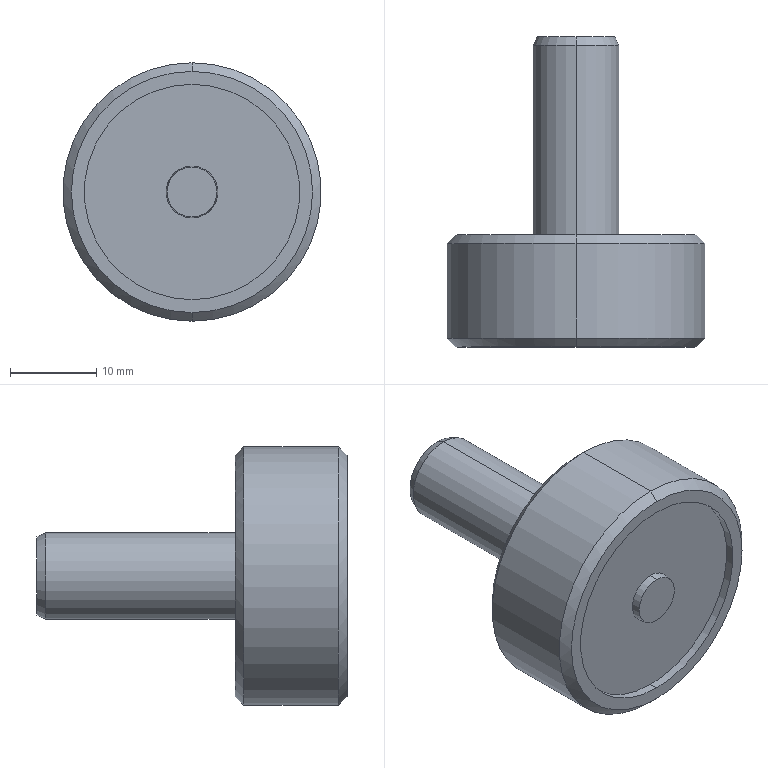Part | SolidWorks | features BaseBody 1 | 1 solid | 19 faces | box 30 x 36 x 30 mm | volume 10433 mm3 | cone 8 | cylinder 6 | plane 5 | commonest cylinder face diameters 10 x2 25 x2 30 x2
STEP:
#1=CARTESIAN_POINT('',(257.5,37.,118.121));
#2=VERTEX_POINT('',#1);
#3=CARTESIAN_POINT('',(257.5,37.,128.121));
#4=VERTEX_POINT('',#3);
#5=CARTESIAN_POINT('',(257.5,37.,123.121));
#6=DIRECTION('',(0.,-1.,0.));
#7=DIRECTION('',(0.,0.,1.));
#8=AXIS2_PLACEMENT_3D('',#5,#6,#7);
#9=CIRCLE('',#8,5.);
#10=EDGE_CURVE('',#2,#4,#9,.T.);
#11=ORIENTED_EDGE('',*,*,#10,.F.);
#12=CARTESIAN_POINT('',(257.5,59.,118.121));
#13=VERTEX_POINT('',#12);
#14=CARTESIAN_POINT('',(257.5,60.,118.121));
#15=DIRECTION('',(0.,1.,0.));
#16=VECTOR('',#15,1000.);
#17=LINE('',#14,#16);
#18=EDGE_CURVE('',#2,#13,#17,.T.);
#19=ORIENTED_EDGE('',*,*,#18,.T.);
#20=CARTESIAN_POINT('',(257.5,59.,128.121));
#21=VERTEX_POINT('',#20);
#22=CARTESIAN_POINT('',(257.5,59.,123.121));
#23=DIRECTION('',(0.,-1.,0.));
#24=DIRECTION('',(0.,0.,1.));
#25=AXIS2_PLACEMENT_3D('',#22,#23,#24);
#26=CIRCLE('',#25,5.);
#27=EDGE_CURVE('',#13,#21,#26,.T.);
#28=ORIENTED_EDGE('',*,*,#27,.T.);
#29=CARTESIAN_POINT('',(257.5,60.,128.121));
#30=DIRECTION('',(0.,1.,0.));
#31=VECTOR('',#30,1000.);
#32=LINE('',#29,#31);
#33=EDGE_CURVE('',#4,#21,#32,.T.);
#34=ORIENTED_EDGE('',*,*,#33,.F.);
#35=EDGE_LOOP('',(#11,#19,#28,#34));
#36=FACE_OUTER_BOUND('',#35,.T.);
#37=CARTESIAN_POINT('',(257.5,60.,123.121));
#38=DIRECTION('',(0.,1.,0.));
#39=DIRECTION('',(0.,0.,1.));
#40=AXIS2_PLACEMENT_3D('',#37,#38,#39);
#41=CYLINDRICAL_SURFACE('',#40,5.);
#42=ADVANCED_FACE('',(#36),#41,.T.);
#43=CARTESIAN_POINT('',(257.5,37.,137.121));
#44=VERTEX_POINT('',#43);
#45=CARTESIAN_POINT('',(257.5,37.,109.121));
#46=VERTEX_POINT('',#45);
#47=CARTESIAN_POINT('',(257.5,37.,123.121));
#48=DIRECTION('',(0.,1.,0.));
#49=DIRECTION('',(0.,0.,-1.));
#50=AXIS2_PLACEMENT_3D('',#47,#48,#49);
#51=CIRCLE('',#50,14.);
#52=EDGE_CURVE('',#44,#46,#51,.T.);
#53=ORIENTED_EDGE('',*,*,#52,.F.);
#54=CARTESIAN_POINT('',(257.5,36.,138.121));
#55=VERTEX_POINT('',#54);
#56=CARTESIAN_POINT('',(257.5,36.,138.121));
#57=DIRECTION('',(0.,-0.7071,0.7071));
#58=VECTOR('',#57,1000.);
#59=LINE('',#56,#58);
#60=EDGE_CURVE('',#44,#55,#59,.T.);
#61=ORIENTED_EDGE('',*,*,#60,.T.);
#62=CARTESIAN_POINT('',(257.5,36.,108.121));
#63=VERTEX_POINT('',#62);
#64=CARTESIAN_POINT('',(257.5,36.,123.121));
#65=DIRECTION('',(0.,1.,0.));
#66=DIRECTION('',(-0.05078,0.,-0.9987));
#67=AXIS2_PLACEMENT_3D('',#64,#65,#66);
#68=CIRCLE('',#67,15.);
#69=EDGE_CURVE('',#55,#63,#68,.T.);
#70=ORIENTED_EDGE('',*,*,#69,.T.);
#71=CARTESIAN_POINT('',(257.5,36.,108.121));
#72=DIRECTION('',(0.,-0.7071,-0.7071));
#73=VECTOR('',#72,1000.);
#74=LINE('',#71,#73);
#75=EDGE_CURVE('',#46,#63,#74,.T.);
#76=ORIENTED_EDGE('',*,*,#75,.F.);
#77=EDGE_LOOP('',(#53,#61,#70,#76));
#78=FACE_OUTER_BOUND('',#77,.T.);
#79=CARTESIAN_POINT('',(257.5,36.,123.121));
#80=DIRECTION('',(0.,-1.,0.));
#81=DIRECTION('',(0.,0.,-1.));
#82=AXIS2_PLACEMENT_3D('',#79,#80,#81);
#83=CONICAL_SURFACE('',#82,15.,0.7854);
#84=ADVANCED_FACE('',(#78),#83,.T.);
#85=CARTESIAN_POINT('',(257.5,60.,118.587));
#86=VERTEX_POINT('',#85);
#87=CARTESIAN_POINT('',(257.5,60.,127.655));
#88=VERTEX_POINT('',#87);
#89=CARTESIAN_POINT('',(257.5,60.,123.121));
#90=DIRECTION('',(0.,-1.,0.));
#91=DIRECTION('',(0.,0.,-1.));
#92=AXIS2_PLACEMENT_3D('',#89,#90,#91);
#93=CIRCLE('',#92,4.534);
#94=EDGE_CURVE('',#86,#88,#93,.T.);
#95=ORIENTED_EDGE('',*,*,#94,.T.);
#96=CARTESIAN_POINT('',(257.5,59.,128.121));
#97=DIRECTION('',(0.,-0.9063,0.4226));
#98=VECTOR('',#97,1000.);
#99=LINE('',#96,#98);
#100=EDGE_CURVE('',#88,#21,#99,.T.);
#101=ORIENTED_EDGE('',*,*,#100,.T.);
#102=ORIENTED_EDGE('',*,*,#27,.F.);
#103=CARTESIAN_POINT('',(257.5,59.,118.121));
#104=DIRECTION('',(0.,-0.9063,-0.4226));
#105=VECTOR('',#104,1000.);
#106=LINE('',#103,#105);
#107=EDGE_CURVE('',#86,#13,#106,.T.);
#108=ORIENTED_EDGE('',*,*,#107,.F.);
#109=EDGE_LOOP('',(#95,#101,#102,#108));
#110=FACE_OUTER_BOUND('',#109,.T.);
#111=CARTESIAN_POINT('',(257.5,59.,123.121));
#112=DIRECTION('',(0.,-1.,0.));
#113=DIRECTION('',(0.,0.,-1.));
#114=AXIS2_PLACEMENT_3D('',#111,#112,#113);
#115=CONICAL_SURFACE('',#114,5.,0.4363);
#116=ADVANCED_FACE('',(#110),#115,.T.);
#117=CARTESIAN_POINT('',(257.5,25.,138.121));
#118=VERTEX_POINT('',#117);
#119=CARTESIAN_POINT('',(257.5,25.,108.121));
#120=VERTEX_POINT('',#119);
#121=CARTESIAN_POINT('',(257.5,25.,123.121));
#122=DIRECTION('',(0.,1.,0.));
#123=DIRECTION('',(0.,0.,1.));
#124=AXIS2_PLACEMENT_3D('',#121,#122,#123);
#125=CIRCLE('',#124,15.);
#126=EDGE_CURVE('',#118,#120,#125,.T.);
#127=ORIENTED_EDGE('',*,*,#126,.T.);
#128=CARTESIAN_POINT('',(257.5,60.,108.121));
#129=DIRECTION('',(0.,1.,0.));
#130=VECTOR('',#129,1000.);
#131=LINE('',#128,#130);
#132=EDGE_CURVE('',#120,#63,#131,.T.);
#133=ORIENTED_EDGE('',*,*,#132,.T.);
#134=ORIENTED_EDGE('',*,*,#69,.F.);
#135=CARTESIAN_POINT('',(257.5,60.,138.121));
#136=DIRECTION('',(0.,1.,0.));
#137=VECTOR('',#136,1000.);
#138=LINE('',#135,#137);
#139=EDGE_CURVE('',#118,#55,#138,.T.);
#140=ORIENTED_EDGE('',*,*,#139,.F.);
#141=EDGE_LOOP('',(#127,#133,#134,#140));
#142=FACE_OUTER_BOUND('',#141,.T.);
#143=CARTESIAN_POINT('',(257.5,60.,123.121));
#144=DIRECTION('',(0.,1.,0.));
#145=DIRECTION('',(0.,0.,1.));
#146=AXIS2_PLACEMENT_3D('',#143,#144,#145);
#147=CYLINDRICAL_SURFACE('',#146,15.);
#148=ADVANCED_FACE('',(#142),#147,.T.);
#149=CARTESIAN_POINT('',(257.5,24.,137.121));
#150=VERTEX_POINT('',#149);
#151=CARTESIAN_POINT('',(257.5,24.,109.121));
#152=VERTEX_POINT('',#151);
#153=CARTESIAN_POINT('',(257.5,24.,123.121));
#154=DIRECTION('',(0.,1.,0.));
#155=DIRECTION('',(0.,0.,1.));
#156=AXIS2_PLACEMENT_3D('',#153,#154,#155);
#157=CIRCLE('',#156,14.);
#158=EDGE_CURVE('',#150,#152,#157,.T.);
#159=ORIENTED_EDGE('',*,*,#158,.T.);
#160=CARTESIAN_POINT('',(257.5,25.,108.121));
#161=DIRECTION('',(0.,0.7071,-0.7071));
#162=VECTOR('',#161,1000.);
#163=LINE('',#160,#162);
#164=EDGE_CURVE('',#152,#120,#163,.T.);
#165=ORIENTED_EDGE('',*,*,#164,.T.);
#166=ORIENTED_EDGE('',*,*,#126,.F.);
#167=CARTESIAN_POINT('',(257.5,25.,138.121));
#168=DIRECTION('',(0.,0.7071,0.7071));
#169=VECTOR('',#168,1000.);
#170=LINE('',#167,#169);
#171=EDGE_CURVE('',#150,#118,#170,.T.);
#172=ORIENTED_EDGE('',*,*,#171,.F.);
#173=EDGE_LOOP('',(#159,#165,#166,#172));
#174=FACE_OUTER_BOUND('',#173,.T.);
#175=CARTESIAN_POINT('',(257.5,25.,123.121));
#176=DIRECTION('',(0.,1.,0.));
#177=DIRECTION('',(0.,0.,1.));
#178=AXIS2_PLACEMENT_3D('',#175,#176,#177);
#179=CONICAL_SURFACE('',#178,15.,0.7854);
#180=ADVANCED_FACE('',(#174),#179,.T.);
#181=CARTESIAN_POINT('',(257.5,25.,135.621));
#182=VERTEX_POINT('',#181);
#183=CARTESIAN_POINT('',(257.5,25.,110.621));
#184=VERTEX_POINT('',#183);
#185=CARTESIAN_POINT('',(257.5,25.,123.121));
#186=DIRECTION('',(0.,-1.,0.));
#187=DIRECTION('',(0.,0.,-1.));
#188=AXIS2_PLACEMENT_3D('',#185,#186,#187);
#189=CIRCLE('',#188,12.5);
#190=EDGE_CURVE('',#182,#184,#189,.T.);
#191=ORIENTED_EDGE('',*,*,#190,.F.);
#192=CARTESIAN_POINT('',(257.5,24.,135.621));
#193=VERTEX_POINT('',#192);
#194=CARTESIAN_POINT('',(257.5,25.,135.621));
#195=DIRECTION('',(0.,-1.,0.));
#196=VECTOR('',#195,1000.);
#197=LINE('',#194,#196);
#198=EDGE_CURVE('',#182,#193,#197,.T.);
#199=ORIENTED_EDGE('',*,*,#198,.T.);
#200=CARTESIAN_POINT('',(257.5,24.,110.621));
#201=VERTEX_POINT('',#200);
#202=CARTESIAN_POINT('',(257.5,24.,123.121));
#203=DIRECTION('',(0.,1.,0.));
#204=DIRECTION('',(0.,0.,-1.));
#205=AXIS2_PLACEMENT_3D('',#202,#203,#204);
#206=CIRCLE('',#205,12.5);
#207=EDGE_CURVE('',#201,#193,#206,.T.);
#208=ORIENTED_EDGE('',*,*,#207,.F.);
#209=CARTESIAN_POINT('',(257.5,25.,110.621));
#210=DIRECTION('',(0.,-1.,0.));
#211=VECTOR('',#210,1000.);
#212=LINE('',#209,#211);
#213=EDGE_CURVE('',#184,#201,#212,.T.);
#214=ORIENTED_EDGE('',*,*,#213,.F.);
#215=EDGE_LOOP('',(#191,#199,#208,#214));
#216=FACE_OUTER_BOUND('',#215,.T.);
#217=CARTESIAN_POINT('',(257.5,25.,123.121));
#218=DIRECTION('',(0.,-1.,0.));
#219=DIRECTION('',(0.,0.,-1.));
#220=AXIS2_PLACEMENT_3D('',#217,#218,#219);
#221=CYLINDRICAL_SURFACE('',#220,12.5);
#222=ADVANCED_FACE('',(#216),#221,.F.);
#223=CARTESIAN_POINT('',(257.5,24.,126.016));
#224=VERTEX_POINT('',#223);
#225=CARTESIAN_POINT('',(257.5,24.,120.226));
#226=VERTEX_POINT('',#225);
#227=CARTESIAN_POINT('',(257.5,24.,123.121));
#228=DIRECTION('',(0.,1.,0.));
#229=DIRECTION('',(0.,0.,1.));
#230=AXIS2_PLACEMENT_3D('',#227,#228,#229);
#231=CIRCLE('',#230,2.895);
#232=EDGE_CURVE('',#224,#226,#231,.T.);
#233=ORIENTED_EDGE('',*,*,#232,.T.);
#234=CARTESIAN_POINT('',(257.5,25.,120.121));
#235=VERTEX_POINT('',#234);
#236=CARTESIAN_POINT('',(257.5,25.,120.121));
#237=DIRECTION('',(0.,0.9945,-0.1045));
#238=VECTOR('',#237,1000.);
#239=LINE('',#236,#238);
#240=EDGE_CURVE('',#226,#235,#239,.T.);
#241=ORIENTED_EDGE('',*,*,#240,.T.);
#242=CARTESIAN_POINT('',(257.5,25.,126.121));
#243=VERTEX_POINT('',#242);
#244=CARTESIAN_POINT('',(257.5,25.,123.121));
#245=DIRECTION('',(0.,1.,0.));
#246=DIRECTION('',(0.,0.,1.));
#247=AXIS2_PLACEMENT_3D('',#244,#245,#246);
#248=CIRCLE('',#247,3.);
#249=EDGE_CURVE('',#243,#235,#248,.T.);
#250=ORIENTED_EDGE('',*,*,#249,.F.);
#251=CARTESIAN_POINT('',(257.5,25.,126.121));
#252=DIRECTION('',(0.,0.9945,0.1045));
#253=VECTOR('',#252,1000.);
#254=LINE('',#251,#253);
#255=EDGE_CURVE('',#224,#243,#254,.T.);
#256=ORIENTED_EDGE('',*,*,#255,.F.);
#257=EDGE_LOOP('',(#233,#241,#250,#256));
#258=FACE_OUTER_BOUND('',#257,.T.);
#259=CARTESIAN_POINT('',(257.5,25.,123.121));
#260=DIRECTION('',(0.,1.,0.));
#261=DIRECTION('',(0.,0.,1.));
#262=AXIS2_PLACEMENT_3D('',#259,#260,#261);
#263=CONICAL_SURFACE('',#262,3.,0.1047);
#264=ADVANCED_FACE('',(#258),#263,.T.);
#265=CARTESIAN_POINT('',(257.5,37.,123.121));
#266=DIRECTION('',(0.,-1.,0.));
#267=DIRECTION('',(0.,0.,1.));
#268=AXIS2_PLACEMENT_3D('',#265,#266,#267);
#269=CIRCLE('',#268,5.);
#270=EDGE_CURVE('',#4,#2,#269,.T.);
#271=ORIENTED_EDGE('',*,*,#270,.T.);
#272=ORIENTED_EDGE('',*,*,#10,.T.);
#273=EDGE_LOOP('',(#271,#272));
#274=FACE_BOUND('',#273,.T.);
#275=CARTESIAN_POINT('',(257.5,37.,123.121));
#276=DIRECTION('',(0.,1.,0.));
#277=DIRECTION('',(0.,0.,-1.));
#278=AXIS2_PLACEMENT_3D('',#275,#276,#277);
#279=CIRCLE('',#278,14.);
#280=EDGE_CURVE('',#46,#44,#279,.T.);
#281=ORIENTED_EDGE('',*,*,#280,.T.);
#282=ORIENTED_EDGE('',*,*,#52,.T.);
#283=EDGE_LOOP('',(#281,#282));
#284=FACE_OUTER_BOUND('',#283,.T.);
#285=CARTESIAN_POINT('',(258.262,37.,138.102));
#286=DIRECTION('',(0.,1.,0.));
#287=DIRECTION('',(0.,0.,1.));
#288=AXIS2_PLACEMENT_3D('',#285,#286,#287);
#289=PLANE('',#288);
#290=ADVANCED_FACE('',(#274,#284),#289,.T.);
#291=ORIENTED_EDGE('',*,*,#18,.F.);
#292=ORIENTED_EDGE('',*,*,#270,.F.);
#293=ORIENTED_EDGE('',*,*,#33,.T.);
#294=CARTESIAN_POINT('',(257.5,59.,123.121));
#295=DIRECTION('',(0.,-1.,0.));
#296=DIRECTION('',(0.,0.,1.));
#297=AXIS2_PLACEMENT_3D('',#294,#295,#296);
#298=CIRCLE('',#297,5.);
#299=EDGE_CURVE('',#21,#13,#298,.T.);
#300=ORIENTED_EDGE('',*,*,#299,.T.);
#301=EDGE_LOOP('',(#291,#292,#293,#300));
#302=FACE_OUTER_BOUND('',#301,.T.);
#303=CARTESIAN_POINT('',(257.5,60.,123.121));
#304=DIRECTION('',(0.,1.,0.));
#305=DIRECTION('',(0.,0.,1.));
#306=AXIS2_PLACEMENT_3D('',#303,#304,#305);
#307=CYLINDRICAL_SURFACE('',#306,5.);
#308=ADVANCED_FACE('',(#302),#307,.T.);
#309=ORIENTED_EDGE('',*,*,#60,.F.);
#310=ORIENTED_EDGE('',*,*,#280,.F.);
#311=ORIENTED_EDGE('',*,*,#75,.T.);
#312=CARTESIAN_POINT('',(257.5,36.,123.121));
#313=DIRECTION('',(0.,1.,0.));
#314=DIRECTION('',(-0.05078,0.,-0.9987));
#315=AXIS2_PLACEMENT_3D('',#312,#313,#314);
#316=CIRCLE('',#315,15.);
#317=EDGE_CURVE('',#63,#55,#316,.T.);
#318=ORIENTED_EDGE('',*,*,#317,.T.);
#319=EDGE_LOOP('',(#309,#310,#311,#318));
#320=FACE_OUTER_BOUND('',#319,.T.);
#321=CARTESIAN_POINT('',(257.5,36.,123.121));
#322=DIRECTION('',(0.,-1.,0.));
#323=DIRECTION('',(0.,0.,-1.));
#324=AXIS2_PLACEMENT_3D('',#321,#322,#323);
#325=CONICAL_SURFACE('',#324,15.,0.7854);
#326=ADVANCED_FACE('',(#320),#325,.T.);
#327=ORIENTED_EDGE('',*,*,#100,.F.);
#328=CARTESIAN_POINT('',(257.5,60.,123.121));
#329=DIRECTION('',(0.,-1.,0.));
#330=DIRECTION('',(0.,0.,-1.));
#331=AXIS2_PLACEMENT_3D('',#328,#329,#330);
#332=CIRCLE('',#331,4.534);
#333=EDGE_CURVE('',#88,#86,#332,.T.);
#334=ORIENTED_EDGE('',*,*,#333,.T.);
#335=ORIENTED_EDGE('',*,*,#107,.T.);
#336=ORIENTED_EDGE('',*,*,#299,.F.);
#337=EDGE_LOOP('',(#327,#334,#335,#336));
#338=FACE_OUTER_BOUND('',#337,.T.);
#339=CARTESIAN_POINT('',(257.5,59.,123.121));
#340=DIRECTION('',(0.,-1.,0.));
#341=DIRECTION('',(0.,0.,-1.));
#342=AXIS2_PLACEMENT_3D('',#339,#340,#341);
#343=CONICAL_SURFACE('',#342,5.,0.4363);
#344=ADVANCED_FACE('',(#338),#343,.T.);
#345=ORIENTED_EDGE('',*,*,#132,.F.);
#346=CARTESIAN_POINT('',(257.5,25.,123.121));
#347=DIRECTION('',(0.,1.,0.));
#348=DIRECTION('',(0.,0.,1.));
#349=AXIS2_PLACEMENT_3D('',#346,#347,#348);
#350=CIRCLE('',#349,15.);
#351=EDGE_CURVE('',#120,#118,#350,.T.);
#352=ORIENTED_EDGE('',*,*,#351,.T.);
#353=ORIENTED_EDGE('',*,*,#139,.T.);
#354=ORIENTED_EDGE('',*,*,#317,.F.);
#355=EDGE_LOOP('',(#345,#352,#353,#354));
#356=FACE_OUTER_BOUND('',#355,.T.);
#357=CARTESIAN_POINT('',(257.5,60.,123.121));
#358=DIRECTION('',(0.,1.,0.));
#359=DIRECTION('',(0.,0.,1.));
#360=AXIS2_PLACEMENT_3D('',#357,#358,#359);
#361=CYLINDRICAL_SURFACE('',#360,15.);
#362=ADVANCED_FACE('',(#356),#361,.T.);
#363=ORIENTED_EDGE('',*,*,#94,.F.);
#364=ORIENTED_EDGE('',*,*,#333,.F.);
#365=EDGE_LOOP('',(#363,#364));
#366=FACE_OUTER_BOUND('',#365,.T.);
#367=CARTESIAN_POINT('',(257.754,60.,128.115));
#368=DIRECTION('',(0.,1.,0.));
#369=DIRECTION('',(0.,0.,1.));
#370=AXIS2_PLACEMENT_3D('',#367,#368,#369);
#371=PLANE('',#370);
#372=ADVANCED_FACE('',(#366),#371,.T.);
#373=ORIENTED_EDGE('',*,*,#164,.F.);
#374=CARTESIAN_POINT('',(257.5,24.,123.121));
#375=DIRECTION('',(0.,1.,0.));
#376=DIRECTION('',(0.,0.,1.));
#377=AXIS2_PLACEMENT_3D('',#374,#375,#376);
#378=CIRCLE('',#377,14.);
#379=EDGE_CURVE('',#152,#150,#378,.T.);
#380=ORIENTED_EDGE('',*,*,#379,.T.);
#381=ORIENTED_EDGE('',*,*,#171,.T.);
#382=ORIENTED_EDGE('',*,*,#351,.F.);
#383=EDGE_LOOP('',(#373,#380,#381,#382));
#384=FACE_OUTER_BOUND('',#383,.T.);
#385=CARTESIAN_POINT('',(257.5,25.,123.121));
#386=DIRECTION('',(0.,1.,0.));
#387=DIRECTION('',(0.,0.,1.));
#388=AXIS2_PLACEMENT_3D('',#385,#386,#387);
#389=CONICAL_SURFACE('',#388,15.,0.7854);
#390=ADVANCED_FACE('',(#384),#389,.T.);
#391=ORIENTED_EDGE('',*,*,#158,.F.);
#392=ORIENTED_EDGE('',*,*,#379,.F.);
#393=EDGE_LOOP('',(#391,#392));
#394=FACE_OUTER_BOUND('',#393,.T.);
#395=ORIENTED_EDGE('',*,*,#207,.T.);
#396=CARTESIAN_POINT('',(257.5,24.,123.121));
#397=DIRECTION('',(0.,1.,0.));
#398=DIRECTION('',(0.,0.,-1.));
#399=AXIS2_PLACEMENT_3D('',#396,#397,#398);
#400=CIRCLE('',#399,12.5);
#401=EDGE_CURVE('',#193,#201,#400,.T.);
#402=ORIENTED_EDGE('',*,*,#401,.T.);
#403=EDGE_LOOP('',(#395,#402));
#404=FACE_BOUND('',#403,.T.);
#405=CARTESIAN_POINT('',(257.5,24.,123.121));
#406=DIRECTION('',(0.,-1.,0.));
#407=DIRECTION('',(0.,0.,-1.));
#408=AXIS2_PLACEMENT_3D('',#405,#406,#407);
#409=PLANE('',#408);
#410=ADVANCED_FACE('',(#394,#404),#409,.T.);
#411=ORIENTED_EDGE('',*,*,#198,.F.);
#412=CARTESIAN_POINT('',(257.5,25.,123.121));
#413=DIRECTION('',(0.,-1.,0.));
#414=DIRECTION('',(0.,0.,-1.));
#415=AXIS2_PLACEMENT_3D('',#412,#413,#414);
#416=CIRCLE('',#415,12.5);
#417=EDGE_CURVE('',#184,#182,#416,.T.);
#418=ORIENTED_EDGE('',*,*,#417,.F.);
#419=ORIENTED_EDGE('',*,*,#213,.T.);
#420=ORIENTED_EDGE('',*,*,#401,.F.);
#421=EDGE_LOOP('',(#411,#418,#419,#420));
#422=FACE_OUTER_BOUND('',#421,.T.);
#423=CARTESIAN_POINT('',(257.5,25.,123.121));
#424=DIRECTION('',(0.,-1.,0.));
#425=DIRECTION('',(0.,0.,-1.));
#426=AXIS2_PLACEMENT_3D('',#423,#424,#425);
#427=CYLINDRICAL_SURFACE('',#426,12.5);
#428=ADVANCED_FACE('',(#422),#427,.F.);
#429=ORIENTED_EDGE('',*,*,#249,.T.);
#430=CARTESIAN_POINT('',(257.5,25.,123.121));
#431=DIRECTION('',(0.,1.,0.));
#432=DIRECTION('',(0.,0.,1.));
#433=AXIS2_PLACEMENT_3D('',#430,#431,#432);
#434=CIRCLE('',#433,3.);
#435=EDGE_CURVE('',#235,#243,#434,.T.);
#436=ORIENTED_EDGE('',*,*,#435,.T.);
#437=EDGE_LOOP('',(#429,#436));
#438=FACE_BOUND('',#437,.T.);
#439=ORIENTED_EDGE('',*,*,#417,.T.);
#440=ORIENTED_EDGE('',*,*,#190,.T.);
#441=EDGE_LOOP('',(#439,#440));
#442=FACE_OUTER_BOUND('',#441,.T.);
#443=CARTESIAN_POINT('',(257.5,25.,123.121));
#444=DIRECTION('',(0.,-1.,0.));
#445=DIRECTION('',(0.,0.,-1.));
#446=AXIS2_PLACEMENT_3D('',#443,#444,#445);
#447=PLANE('',#446);
#448=ADVANCED_FACE('',(#438,#442),#447,.T.);
#449=ORIENTED_EDGE('',*,*,#240,.F.);
#450=CARTESIAN_POINT('',(257.5,24.,123.121));
#451=DIRECTION('',(0.,1.,0.));
#452=DIRECTION('',(0.,0.,1.));
#453=AXIS2_PLACEMENT_3D('',#450,#451,#452);
#454=CIRCLE('',#453,2.895);
#455=EDGE_CURVE('',#226,#224,#454,.T.);
#456=ORIENTED_EDGE('',*,*,#455,.T.);
#457=ORIENTED_EDGE('',*,*,#255,.T.);
#458=ORIENTED_EDGE('',*,*,#435,.F.);
#459=EDGE_LOOP('',(#449,#456,#457,#458));
#460=FACE_OUTER_BOUND('',#459,.T.);
#461=CARTESIAN_POINT('',(257.5,25.,123.121));
#462=DIRECTION('',(0.,1.,0.));
#463=DIRECTION('',(0.,0.,1.));
#464=AXIS2_PLACEMENT_3D('',#461,#462,#463);
#465=CONICAL_SURFACE('',#464,3.,0.1047);
#466=ADVANCED_FACE('',(#460),#465,.T.);
#467=ORIENTED_EDGE('',*,*,#232,.F.);
#468=ORIENTED_EDGE('',*,*,#455,.F.);
#469=EDGE_LOOP('',(#467,#468));
#470=FACE_OUTER_BOUND('',#469,.T.);
#471=CARTESIAN_POINT('',(257.5,24.,123.121));
#472=DIRECTION('',(0.,-1.,0.));
#473=DIRECTION('',(0.,0.,-1.));
#474=AXIS2_PLACEMENT_3D('',#471,#472,#473);
#475=PLANE('',#474);
#476=ADVANCED_FACE('',(#470),#475,.T.);
#477=CLOSED_SHELL('',(#42,#84,#116,#148,#180,#222,#264,#290,#308,#326,#344,#362,#372,#390,#410,#428,#448,#466,#476));
#478=MANIFOLD_SOLID_BREP('',#477);
#479=CARTESIAN_POINT('',(0.,0.,0.));
#480=DIRECTION('',(0.,0.,1.));
#481=DIRECTION('',(1.,0.,0.));
#482=AXIS2_PLACEMENT_3D('',#479,#480,#481);
#483=(LENGTH_UNIT()NAMED_UNIT(*)SI_UNIT(.MILLI.,.METRE.));
#484=UNCERTAINTY_MEASURE_WITH_UNIT(LENGTH_MEASURE(0.00001),#483,'','');
#485=(NAMED_UNIT(*)PLANE_ANGLE_UNIT()SI_UNIT($,.RADIAN.));
#486=(NAMED_UNIT(*)SI_UNIT($,.STERADIAN.)SOLID_ANGLE_UNIT());
#487=(GEOMETRIC_REPRESENTATION_CONTEXT(3)GLOBAL_UNCERTAINTY_ASSIGNED_CONTEXT((#484))GLOBAL_UNIT_ASSIGNED_CONTEXT((#483,#485,#486))REPRESENTATION_CONTEXT('',''));
#488=ADVANCED_BREP_SHAPE_REPRESENTATION('',(#478,#482),#487);